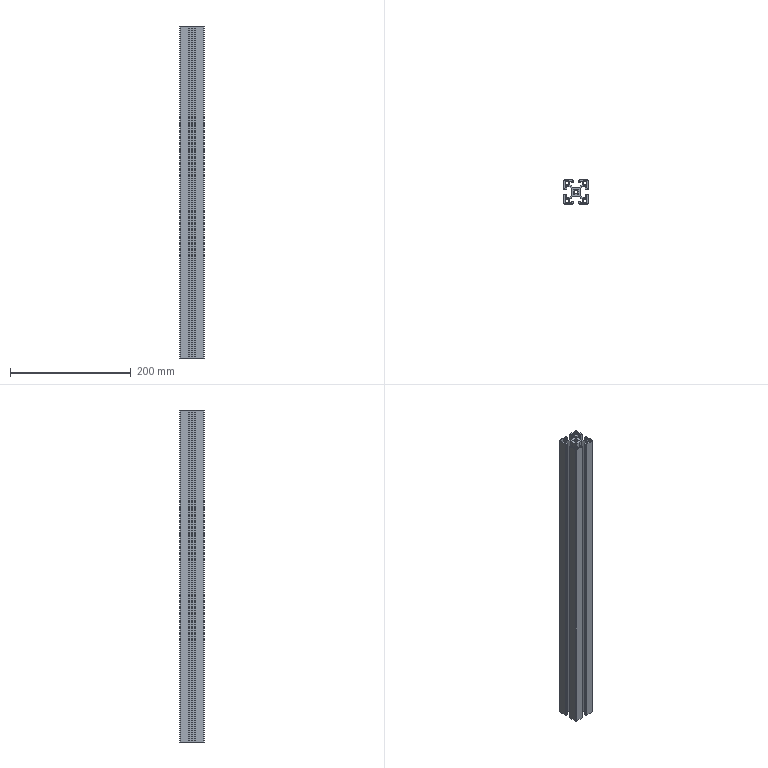Part | NX | features BREP 1 | 1 solid | 161 faces | box 40 x 40 x 550 mm | volume 334454 mm3 | plane 114 | cylinder 47 | commonest cylinder face diameters 0.6 x16 1 x8 2 x8 1.5 x6 6.8 x5 3 x4